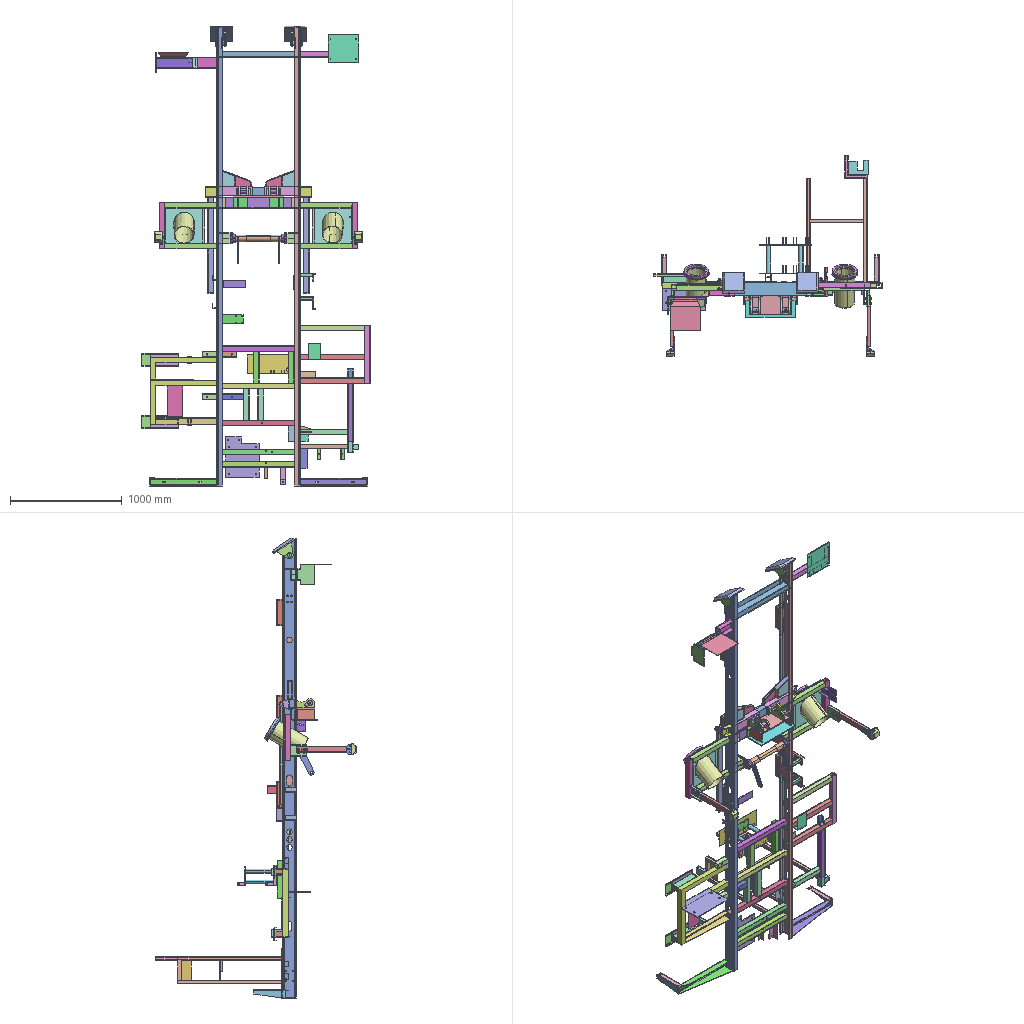Assembly | SolidWorks | 152 different items | 310 placed | box 2045 x 1800 x 4124 mm
Parts list (item | name | quantity | parent item | size | volume | features):
1 | (subassembly) | x1 | - | 650 x 415 x 555 mm | 2554189 mm3 | -
2 | (subassembly) | x1 | - | 625 x 50 x 1040 mm | 1628220 mm3 | -
3 | (subassembly) | x2 | in 20 | 255 x 100 x 75 mm | 251400 mm3 | -
4 | (subassembly) | x1 | - | 75 x 280 x 45 mm | 137505 mm3 | -
5 | (subassembly) | x1 | - | 75 x 280 x 45 mm | 137505 mm3 | -
6 | (subassembly) | x2 | - | 100 x 145 x 100 mm | 200705 mm3 | -
7 | (subassembly) | x1 | - | 320 x 140 x 260 mm | 518000 mm3 | -
8 | (subassembly) | x6 | - | 50 x 55 x 340 mm | 668931 mm3 | -
9 | (subassembly) | x1 | - | 470 x 410 x 340 mm | 1561972 mm3 | features CompositeCurve 1
10 | (subassembly) | x8 | in 12 | 30 x 70 x 30 mm | 19249 mm3 | -
11 | (subassembly) | x1 | - | 100 x 120 x 206 mm | 195480 mm3 | -
12 | (subassembly) | x2 | in 9 | 470 x 170 x 75 mm | 476496 mm3 | -
13 | (subassembly) | x2 | - | 220 x 200 x 152.25 mm | 1422788 mm3 | -
14 | (subassembly) | x1 | - | 740 x 271 x 356.521 mm | 7282688 mm3 | -
15 | (subassembly) | x1 | - | 100 x 120 x 186 mm | 156515 mm3 | -
16 | (subassembly) | x1 | in 1 | 115 x 70 x 590 mm | 694162 mm3 | -
17 | (subassembly) | x1 | - | 115 x 70 x 590 mm | 694162 mm3 | -
18 | (subassembly) | x1 | - | 240 x 550.386 x 1140 mm | 2006489 mm3 | -
19 | (subassembly) | x1 | - | 250 x 58 x 520 mm | 854172 mm3 | -
20 | (subassembly) | x1 | - | 670 x 679 x 350 mm | 6681569 mm3 | -
21 | (subassembly) | x1 | - | 183 x 366.464 x 548.536 mm | 871014 mm3 | -
22 | (subassembly) | x2 | - | 100.467 x 200 x 740 mm | 967974 mm3 | -
23 | (subassembly) | x3 | in 1 | 230 x 230 x 340 mm | 1372483 mm3 | -
24 | (subassembly) | x1 | - | 60 x 415 x 515 mm | 1791277 mm3 | -
25 | - | x2 | in 18 | 30 x 30 x 100 mm | 16864 mm3 | features Extrusion 1, ICE 1
26 | - | x1 | in 21 | 43 x 310 x 270 mm | 250121 mm3 | features Extrusion 1, ICE 1
27 | - | x1 | in 20 | 140 x 280 x 83 mm | 150930 mm3 | features Extrusion 1, Fillet 1, ICE 1
28 | - | x1 | in 20 | 390 x 250 x 8 mm | 755753 mm3 | features ICE 2, Extrusion 1
29 | - | x2 | in 11, 15 | 100 x 120 x 6 mm | 72000 mm3 | features Extrusion 1
30 | - | x1 | in 15 | 180 x 80 x 6 mm | 84515 mm3 | features Extrusion 1, ICE 1
31 | - | x2 | in 20 | 70 x 30 x 100 mm | 55604 mm3 | features Extrusion 1, ICE 1, Shell 1
32 | - | x1 | - | 50 x 120 x 4120 mm | 4129242 mm3 | features ICE 5, Cut 2, Extrusion 1
33 | - | x1 | - | 50 x 120 x 4120 mm | 4181068 mm3 | features ICE 4, Cut 2, Extrusion 1
34 | - | x1 | - | 60 x 60 x 470 mm | 1026298 mm3 | features ICE 2, RevCut 2, Extrusion 1
35 | - | x2 | - | 75 x 75 x 25 mm | 32210 mm3 | features Chamfer 1, Extrusion 1, ICE 1
36 | - | x1 | - | 50 x 50 x 160 mm | 46324 mm3 | features Extrusion 1, ICE 1
37 | - | x2 | - | 25 x 25 x 90 mm | 18731 mm3 | features ICE 4, Chamfer 3, Extrusion 1
38 | - | x2 | - | 77.5 x 50 x 90 mm | 116974 mm3 | features ICE 3, Extrusion 1
39 | - | x2 | - | 67.801 x 45 x 103 mm | 100967 mm3 | features ICE 3, Extrusion 1
40 | - | x2 | in 16, 17 | 105 x 30 x 140 mm | 154453 mm3 | features Extrusion 1, ICE 1
41 | - | x2 | in 16, 17 | 50 x 30 x 450 mm | 193179 mm3 | features ICE 2, Extrusion 1
42 | - | x2 | in 16, 17 | 90 x 135 x 60 mm | 111719 mm3 | features ICE 6, Extrusion 1
43 | - | x2 | in 16, 17 | 100 x 40 x 70 mm | 234811 mm3 | features Extrusion 1, Fillet 1
44 | - | x2 | - | 243.637 x 59.938 x 8 mm | 90831 mm3 | features Extrusion 1, ICE 1
45 | - | x4 | in 14 | 85.082 x 170 x 15 mm | 155113 mm3 | features ICE 3, Extrusion 1
46 | - | x2 | - | 50 x 50 x 280 mm | 157920 mm3 | features Extrusion 1
47 | - | x1 | - | 30 x 30 x 100 mm | 11600 mm3 | features Extrusion 1
48 | - | x1 | - | 50 x 50 x 130 mm | 72524 mm3 | features Cut 1, Extrusion 1
49 | - | x1 | - | 50 x 50 x 190 mm | 106364 mm3 | features Cut 1, Extrusion 1
50 | - | x2 | - | 50 x 50 x 130 mm | 72524 mm3 | features Cut 1, Extrusion 1
51 | - | x2 | - | 45 x 45 x 50 mm | 31416 mm3 | features ICE 2, Extrusion 1
52 | - | x4 | - | 57.32 x 20.473 x 17.73 mm | 7614 mm3 | features RevCut 3, Boss 1, Chamfer 1, Extrusion 1, Fillet 1, LPattern 1
53 | - | x4 | - | 41.4 x 18.475 x 16 mm | 4135 mm3 | features RevCut 3, Boss 1, Chamfer 1, Extrusion 1, Fillet 1, LPattern 1
54 | - | x4 | - | 20.785 x 18 x 10.8 mm | 1984 mm3 | features RevCut 2, Chamfer 1, Extrusion 1, LPattern 1
55 | - | x8 | - | 37.68 x 20.473 x 17.73 mm | 5450 mm3 | features RevCut 3, Boss 1, Chamfer 1, Extrusion 1, Fillet 1, LPattern 1
56 | - | x4 | - | 24 x 24 x 2.5 mm | 799.143 mm3 | features Extrusion 1
57 | - | x4 | - | 50 x 50 x 10 mm | 24215 mm3 | features Extrusion 1
58 | - | x1 | - | 595 x 120 x 70 mm | 542052 mm3 | features ICE 3, Fillet 2, Extrusion 1, Shell 1
59 | - | x1 | - | 595 x 120 x 70 mm | 542052 mm3 | features ICE 3, Fillet 2, Extrusion 1, Shell 1
60 | - | x1 | in 19 | 50 x 50 x 520 mm | 293280 mm3 | features Extrusion 1
61 | - | x1 | in 19 | 270 x 250 x 8 mm | 538392 mm3 | features Cut 1, Extrusion 1
62 | - | x4 | in 19 | 100 x 30 x 5 mm | 7500 mm3 | features Extrusion 1
63 | - | x2 | in 19 | 50 x 30 x 5 mm | 3750 mm3 | features Extrusion 1
64 | - | x1 | in 14 | 90 x 600 x 5 mm | 270000 mm3 | features Extrusion 1, ICE 1
65 | - | x1 | - | 50 x 180 x 10 mm | 87345 mm3 | features Extrusion 1, ICE 1
66 | - | x1 | - | 60 x 140 x 8 mm | 67200 mm3 | features Extrusion 1
67 | - | x1 | in 20 | 595 x 605 x 50 mm | 4237500 mm3 | features ICE 10, Cut 1, Extrusion 1
68 | - | x1 | in 20 | 545 x 80 x 60 mm | 449625 mm3 | features Extrusion 1, ICE 1, Shell 1
69 | - | x1 | - | 45 x 110 x 79.839 mm | 29548 mm3 | features Extrusion 1, ICE 1
70 | - | x1 | - | 79.839 x 110 x 45 mm | 29548 mm3 | features Fillet 2, Extrusion 1
71 | - | x1 | - | 53 x 120 x 740 mm | 751500 mm3 | features ICE 3, Extrusion 1
72 | - | x1 | in 21 | 100 x 50 x 175 mm | 166250 mm3 | features Extrusion 1
73 | - | x1 | in 21 | 43.536 x 90 x 100 mm | 52249 mm3 | features ICE 2, Extrusion 1
74 | - | x1 | in 21 | 70.878 x 56.464 x 5 mm | 9823 mm3 | features Extrusion 1, ICE 1
75 | - | x1 | - | 120 x 120 x 10 mm | 138691 mm3 | features Extrusion 1
76 | - | x1 | in 21 | 100 x 30 x 360 mm | 264321 mm3 | features Extrusion 1, ICE 1
77 | - | x2 | in 22 | 50 x 120 x 125 mm | 108750 mm3 | features Cut 3, Extrusion 1, ICE 1
78 | - | x6 | in 22 | 50 x 120 x 125 mm | 108750 mm3 | features Cut 3, Extrusion 1, ICE 1
79 | - | x6 | in 22 | 90 x 110 x 10 mm | 91931 mm3 | features ICE 2, Extrusion 1
80 | - | x4 | in 22 | 100 x 200 x 10 mm | 174555 mm3 | features ICE 4, Extrusion 1
81 | - | x3 | in 23 | 180 x 180 x 320 mm | 879646 mm3 | features Extrusion 1
82 | - | x3 | in 23 | 230 x 230 x 15 mm | 115846 mm3 | features ICE 5, Cut 1, Extrusion 1
83 | - | x4 | in 1, 24 | 50 x 50 x 465 mm | 262260 mm3 | features Extrusion 1
84 | - | x2 | in 1, 24 | 50 x 50 x 415 mm | 234060 mm3 | features Extrusion 1
85 | - | x2 | in 1, 24 | 400 x 365 x 5 mm | 558599 mm3 | features Extrusion 1, ICE 1
86 | - | x1 | in 11 | 200 x 100 x 70 mm | 123480 mm3 | features Extrusion 1
87 | - | x2 | in 1, 24 | 380 x 330 x 5 mm | 474099 mm3 | features Cut 1, Extrusion 1, ICE 1
88 | - | x2 | in 14 | 100 x 120 x 10 mm | 120000 mm3 | features ICE 3, Extrusion 1
89 | - | x1 | - | 100 x 50 x 100 mm | 84600 mm3 | features ICE 3, Extrusion 1
90 | - | x2 | - | 110 x 100 x 5 mm | 38408 mm3 | features ICE 5, Extrusion 1
91 | - | x2 | - | 65 x 65 x 50 mm | 86394 mm3 | features Extrusion 1
92 | - | x1 | in 7 | 70 x 30 x 260 mm | 185360 mm3 | features Cut 1, Extrusion 1
93 | - | x1 | in 7 | 110 x 30 x 180 mm | 190080 mm3 | features Extrusion 1
94 | - | x4 | in 7 | 30 x 30 x 110 mm | 35640 mm3 | features Cut 1, Extrusion 1
95 | - | x1 | in 1 | 130 x 180 x 28 mm | 68749 mm3 | features ICE 2, Extrusion 1
96 | - | x1 | in 2 | 50 x 50 x 520 mm | 293280 mm3 | features Cut 1, Extrusion 1, ICE 1
97 | - | x1 | in 18 | 240 x 540 x 940 mm | 1507680 mm3 | features ICE 4, Extrusion 1
98 | - | x1 | in 2 | 50 x 50 x 425 mm | 239700 mm3 | features Cut 1, Extrusion 1, ICE 1
99 | - | x2 | in 2 | 50 x 50 x 575 mm | 324300 mm3 | features Cut 1, Extrusion 1
100 | - | x1 | in 2 | 80 x 50 x 50 mm | 27360 mm3 | features Extrusion 1, Shell 1
101 | - | x1 | in 2 | 170 x 60 x 8 mm | 78676 mm3 | features Extrusion 1, ICE 1
102 | - | x1 | in 2 | 50 x 50 x 520 mm | 293280 mm3 | features ICE 2, Extrusion 1
103 | - | x1 | in 2 | 50 x 50 x 575 mm | 324300 mm3 | features Extrusion 1, ICE 1
104 | - | x1 | in 2 | 60 x 70 x 10 mm | 42000 mm3 | features Extrusion 1
105 | - | x1 | in 2 | 140 x 60 x 10 mm | 84000 mm3 | features Extrusion 1
106 | - | x4 | in 3 | 255 x 70 x 3 mm | 53550 mm3 | features Extrusion 1
107 | - | x4 | in 3 | 40 x 70 x 3 mm | 8400 mm3 | features Extrusion 1
108 | - | x1 | in 18 | 80 x 180 x 8 mm | 115200 mm3 | features Extrusion 1
109 | - | x2 | in 3 | 255 x 100 x 5 mm | 127500 mm3 | features ICE 3, Extrusion 1
110 | - | x2 | in 4, 5 | 75 x 280 x 5 mm | 83125 mm3 | features Extrusion 1
111 | - | x2 | in 4, 5 | 8.684 x 279.845 x 40 mm | 54380 mm3 | features ICE 2, Extrusion 1
112 | - | x1 | in 21 | 180 x 155 x 5 mm | 128250 mm3 | features Extrusion 1, ICE 1
113 | - | x2 | - | 54.442 x 50 x 920.099 mm | 408787 mm3 | features ICE 4, Extrusion 1
114 | - | x2 | in 6 | 100 x 60 x 100 mm | 126908 mm3 | features Fillet 2, Extrusion 1, Shell 1
115 | - | x4 | in 6 | 80 x 85 x 8 mm | 36899 mm3 | features Extrusion 1
116 | - | x2 | in 20 | 120 x 20 x 330 mm | 236877 mm3 | features Extrusion 1, ICE 1
117 | - | x1 | in 14 | 80 x 60 x 740 mm | 962000 mm3 | features ICE 6, Cut 2, Extrusion 1
118 | - | x1 | - | 50 x 50 x 740 mm | 402309 mm3 | features ICE 6, Cut 3, Extrusion 1
119 | - | x1 | in 18 | 200 x 30 x 200 mm | 119880 mm3 | features Extrusion 1, ICE 1, Shell 1
120 | - | x1 | - | 50 x 50 x 740 mm | 401838 mm3 | features ICE 11, Cut 4, Extrusion 1
121 | - | x1 | - | 50 x 50 x 740 mm | 402309 mm3 | features ICE 8, Cut 3, Extrusion 1
122 | - | x1 | - | 50 x 50 x 740 mm | 402780 mm3 | features ICE 5, Extrusion 1
123 | - | x1 | - | 50 x 50 x 740 mm | 402780 mm3 | features ICE 5, Extrusion 1
124 | - | x6 | in 8 | 340 x 50 x 5 mm | 85000 mm3 | features Extrusion 1
125 | - | x6 | in 8 | 50 x 50 x 240 mm | 583931 mm3 | features ICE 2, Extrusion 1, Fillet 1
126 | - | x3 | in 23 | 220 x 220 x 30 mm | 376991 mm3 | features Extrusion 1
127 | - | x2 | - | 40 x 40 x 100 mm | 37500 mm3 | features Extrusion 1
128 | - | x2 | in 12 | 470 x 170 x 5 mm | 399500 mm3 | features Extrusion 1
129 | - | x16 | in 10 | 30 x 70 x 5 mm | 9624 mm3 | features Extrusion 1
130 | - | x1 | in 18 | 180 x 130 x 5 mm | 86000 mm3 | features Extrusion 1
131 | - | x2 | in 9 | 50 x 50 x 340 mm | 191760 mm3 | features Extrusion 1
132 | - | x2 | in 9 | 50 x 30 x 170 mm | 53040 mm3 | features Extrusion 1, ICE 1
133 | - | x2 | in 9 | 40 x 40 x 250 mm | 59690 mm3 | features Extrusion 1
134 | - | x1 | - | 300 x 360 x 10 mm | 979288 mm3 | features ICE 2, Extrusion 1
135 | - | x2 | in 13 | 220 x 200 x 30 mm | 1200000 mm3 | features ICE 1, NetBlend 1
136 | - | x4 | in 13 | 160 x 10 x 122.25 mm | 111394 mm3 | features Extrusion 1, ICE 1
137 | - | x2 | in 14 | 154.478 x 150 x 8 mm | 150374 mm3 | features Extrusion 1
138 | - | x2 | in 14 | 88 x 76 x 318 mm | 396864 mm3 | features ICE 3, Extrusion 1
139 | - | x2 | in 14 | 300 x 150 x 8 mm | 227361 mm3 | features Extrusion 1
140 | - | x1 | in 14 | 308 x 158.521 x 50 mm | 106428 mm3 | features Extrusion 1, ICE 1
141 | - | x1 | in 18 | 120 x 240 x 5 mm | 144000 mm3 | features Extrusion 1
142 | - | x1 | in 14 | 308 x 158.521 x 50 mm | 106428 mm3 | features Extrusion 1, ICE 1
143 | - | x2 | in 14 | 320 x 80 x 8 mm | 197260 mm3 | features Extrusion 1, ICE 1
144 | - | x2 | in 14 | 137.522 x 90.425 x 8 mm | 71106 mm3 | features Extrusion 1
145 | - | x2 | in 14 | 8 x 93.358 x 42 mm | 30876 mm3 | features Extrusion 1, ICE 1
146 | - | x4 | in 14 | 150 x 90 x 10 mm | 135000 mm3 | features Extrusion 1
147 | - | x1 | in 14 | 440 x 180 x 10 mm | 792000 mm3 | features Extrusion 1
148 | - | x1 | in 14 | 460 x 240 x 10 mm | 1004000 mm3 | features ICE 2, Extrusion 1
149 | - | x2 | in 14 | 20 x 60 x 10 mm | 12000 mm3 | features ICE 2, Extrusion 1
150 | - | x4 | in 14 | 20 x 70 x 10 mm | 14000 mm3 | features Extrusion 1
151 | - | x1 | - | 150 x 60 x 110 mm | 112750 mm3 | features Extrusion 1
152 | - | x1 | in 14 | 100 x 48 x 740 mm | 683700 mm3 | features ICE 6, Cut 4, Extrusion 1
Mates (type | each side: item.copy, entity, surface, feature):
In the top assembly
Coincident | 32.1 face plane Boss-Extrude 1 | 33.1 face plane Boss-Extrude 1 | 2 times
Coincident | 32.1 face plane Boss-Extrude 1 | 118.1 face plane Cut-Extrude 1
Coincident | 118.1 face plane Boss-Extrude 1 | 36.1 face plane Boss-Extrude 1 | 2 times
DistanceDim | 118.1 face plane Boss-Extrude 1 | 32.1 face plane Boss-Extrude 1
Coincident | 36.1 face plane Boss-Extrude 1 | 57.1 face plane Boss-Extrude 1
Concentric | 36.1 face cylinder Cut-Extrude 1 | 57.1 face cylinder Boss-Extrude 1
Parallel | 36.1 face plane Boss-Extrude 1 | 57.1 face plane Boss-Extrude 1
DistanceDim | 36.1 face plane Boss-Extrude 1 | 32.1 face plane Boss-Extrude 1
Coincident | 118.1 face plane Boss-Extrude 1 | 47.1 face plane Boss-Extrude 2 | 2 times
DistanceDim | 57.2 face plane Boss-Extrude 1 | 32.1 face plane Boss-Extrude 1
Coincident | 32.1 face plane Boss-Extrude 1 | 57.3 face plane Boss-Extrude 1 | 2 times
Coincident | 118.1 face plane Boss-Extrude 1 | 134.1 face plane Boss-Extrude 1
Coincident | 32.1 face plane Boss-Extrude 1 | 120.1 face plane Cut-Extrude 1
DistanceDim | 120.1 face plane Boss-Extrude 1 | 118.1 face plane Boss-Extrude 1
Coincident | 57.3 face plane Boss-Extrude 1 | 120.1 face plane Boss-Extrude 1
Coincident | 57.2 face plane Boss-Extrude 1 | 120.1 face plane Boss-Extrude 1 | 2 times
DistanceDim | 47.1 face plane Boss-Extrude 2 | 32.1 face plane Boss-Extrude 1
DistanceDim | 134.1 face plane Boss-Extrude 1 | 33.1 face plane Boss-Extrude 1 | 2 times
Coincident | 32.1 face plane Boss-Extrude 1 | 121.1 face plane Cut-Extrude 1
DistanceDim | 120.1 face plane Boss-Extrude 1 | 121.1 face plane Boss-Extrude 1
Coincident | 121.1 face plane Boss-Extrude 1 | 57.4 face plane Boss-Extrude 1
Concentric | 121.1 face cylinder Cut-Extrude 3 | 57.4 face cylinder Boss-Extrude 1
Coincident | 121.1 face plane Boss-Extrude 1 | 66.1 face plane Boss-Extrude 1 | 2 times
Coincident | 32.1 face plane Boss-Extrude 1 | 66.1 face plane Boss-Extrude 1
Coincident | 32.1 face plane Boss-Extrude 1 | 122.1 face plane Cut-Extrude 1
Coincident | 32.1 edge | 122.1 face plane Cut-Extrude 1
DistanceDim | 121.1 face plane Boss-Extrude 1 | 122.1 face plane Boss-Extrude 1
Coincident | 32.1 face plane Boss-Extrude 1 | 123.1 face plane Cut-Extrude 1 | 2 times
DistanceDim | 123.1 face plane Boss-Extrude 1 | 122.1 face plane Boss-Extrude 1
Coincident | 121.1 face plane Boss-Extrude 1 | 46.1 face plane Boss-Extrude 2 | 2 times
Coincident | 122.1 face plane Boss-Extrude 1 | 46.2 face plane Boss-Extrude 2
DistanceDim | 46.1 face plane Boss-Extrude 2 | 33.1 face plane Boss-Extrude 1
DistanceDim | 46.2 face plane Boss-Extrude 2 | 46.1 face plane Boss-Extrude 2
Coincident | 46.1 face plane Boss-Extrude 2 | 49.1 face plane Boss-Extrude 2 | 2 times
Coincident | 33.1 face plane Boss-Extrude 1 | 48.1 face plane Boss-Extrude 1
Coincident | 123.1 face plane Boss-Extrude 1 | 48.1 face plane Boss-Extrude 1 | 2 times
DistanceDim | 49.1 select_type:24 | 48.1 select_type:24
Coincident | 32.1 face plane Boss-Extrude 1 | 121.1 face plane Cut-Extrude 6
Coincident | 121.1 face plane Boss-Extrude 1 | 46.2 face plane Boss-Extrude 2
Coincident | 33.1 face plane Boss-Extrude 1 | 120.1 face plane Boss-Extrude 2
Coincident | 33.1 face plane Boss-Extrude 1 | 121.1 face plane Boss-Extrude 4
Coincident | 32.1 face plane Boss-Extrude 1 | 118.1 face plane Cut-Extrude 6
Coincident | 33.1 face plane Boss-Extrude 1 | 50.1 face plane Boss-Extrude 1
Coincident | 122.1 face plane Boss-Extrude 1 | 50.1 face plane Boss-Extrude 1
Coincident | 49.1 face plane Boss-Extrude 2 | 50.1 face plane Boss-Extrude 1
Coincident | 33.1 face plane Boss-Extrude 1 | 50.2 face plane Boss-Extrude 1
Coincident | 46.2 face plane Boss-Extrude 2 | 65.1 face plane Boss-Extrude 1 | 2 times
DistanceDim | 65.1 face plane Boss-Extrude 1 | 121.1 face plane Boss-Extrude 1
Coincident | 32.1 face plane Boss-Extrude 1 | 152.1 face plane Cut-Extrude 2
Coincident | 32.1 face plane Boss-Extrude 1 | 152.1 face plane Boss-Extrude 4
Coincident | 152.1 face plane Boss-Extrude 1 | assembly select_type:11
Coincident | 33.1 face plane Boss-Extrude 1 | 29.1 face plane Boss-Extrude 1 | 2 times
DistanceDim | 29.1 face plane Boss-Extrude 1 | 123.1 face plane Boss-Extrude 1
Coincident | 33.1 face plane Boss-Extrude 1 | 29.2 face plane Boss-Extrude 1 | 2 times
DistanceDim | 29.2 face plane Boss-Extrude 1 | 123.1 face plane Boss-Extrude 1
Coincident | 32.1 face plane Boss-Extrude 1 | 75.1 face plane Boss-Extrude 1 | 2 times
DistanceDim | 75.1 face plane Boss-Extrude 1 | 123.1 edge
Coincident | 33.1 face plane Boss-Extrude 1 | 78.1 face plane Cut-Extrude 1
Coincident | 32.1 face plane Boss-Extrude 1 | 77.1 face plane Cut-Extrude 1
Coincident | 78.1 face plane Boss-Extrude 1 | 77.1 face plane Boss-Extrude 1
Coincident | 32.1 face plane Boss-Extrude 1 | 71.1 face plane Cut-Extrude 3
Coincident | 33.1 face plane Boss-Extrude 1 | 71.1 face plane Boss-Extrude 1
DistanceDim | 71.1 face plane Boss-Extrude 1 | 32.1 face plane Boss-Extrude 1
Coincident | 48.1 face plane Boss-Extrude 1 | 50.2 face plane Boss-Extrude 1 | 2 times
Coincident | 88.1 face plane Boss-Extrude 1 | 146.1 face plane Boss-Extrude 1
Coincident | 148.1 face plane Boss-Extrude 2 | 146.1 face plane Boss-Extrude 1
Coincident | 148.1 face plane Boss-Extrude 1 | 146.1 face plane Boss-Extrude 1
Coincident | 88.2 face plane Boss-Extrude 1 | 146.2 face plane Boss-Extrude 1
Coincident | 148.1 face plane Boss-Extrude 1 | 146.2 face plane Boss-Extrude 1
Coincident | 148.1 face plane Boss-Extrude 3 | 146.2 face plane Boss-Extrude 1
Coincident | 32.1 face plane Boss-Extrude 1 | 98.1 face plane Boss-Extrude 2
Coincident | 33.1 face plane Boss-Extrude 1 | 67.1 face plane Boss-Extrude 9
Coincident | 33.1 face plane Boss-Extrude 1 | 68.1 face plane Boss-Extrude 1
Coincident | 50.2 face plane Boss-Extrude 1 | 67.1 face plane Boss-Extrude 1
Coincident | 32.1 face plane Boss-Extrude 1 | 98.1 face plane Boss-Extrude 1
DistanceDim | 96.1 face plane Cut-Extrude 1 | 32.1 face plane Boss-Extrude 1
Coincident | 33.1 face plane Boss-Extrude 1 | 59.1 face plane Boss-Extrude 1 | 2 times
DistanceDim | 59.1 face plane Boss-Extrude 1 | 33.1 face plane Boss-Extrude 1
Coincident | 32.1 face plane Boss-Extrude 1 | 58.1 face plane Boss-Extrude 1
DistanceDim | 58.1 face plane Boss-Extrude 1 | 32.1 face plane Boss-Extrude 1
Coincident | 58.1 face plane Boss-Extrude 1 | 32.1 face plane Boss-Extrude 1
Coincident | 59.1 face plane Boss-Extrude 1 | 110.1 face plane Boss-Extrude 3
Coincident | 59.1 face plane Boss-Extrude 1 | 111.1 face plane Boss-Extrude 1
Coincident | 59.1 edge | 110.1 face plane Boss-Extrude 3
Coincident | 58.1 face plane Boss-Extrude 1 | 110.2 face plane Boss-Extrude 3
Coincident | 58.1 face plane Boss-Extrude 1 | 111.2 face plane Boss-Extrude 1
Coincident | 58.1 edge | 110.2 face plane Boss-Extrude 3
Coincident | 33.1 face plane Boss-Extrude 1 | 114.1 face plane Boss-Extrude 1
Parallel | 33.1 face plane Boss-Extrude 1 | 114.1 face plane Boss-Extrude 1
DistanceDim | 114.1 face plane Boss-Extrude 1 | 123.1 face plane Boss-Extrude 1
Coincident | 32.1 face plane Boss-Extrude 1 | 114.2 face plane Boss-Extrude 1
DistanceDim | 114.2 face plane Boss-Extrude 1 | 123.1 face plane Boss-Extrude 1
Coincident | 33.1 face plane Boss-Extrude 1 | 124.1 face plane Boss-Extrude 1
Coincident | 33.1 face plane Boss-Extrude 1 | 125.1 face plane Boss-Extrude 2
Coincident | 33.1 face plane Boss-Extrude 1 | 124.2 face plane Boss-Extrude 1 | 2 times
Coincident | 33.1 face plane Boss-Extrude 1 | 124.3 face plane Boss-Extrude 1 | 2 times
Coincident | 32.1 face plane Boss-Extrude 1 | 124.4 face plane Boss-Extrude 1 | 2 times
Coincident | 32.1 face plane Boss-Extrude 1 | 124.5 face plane Boss-Extrude 1 | 2 times
Coincident | 32.1 face plane Boss-Extrude 1 | 124.6 face plane Boss-Extrude 1 | 2 times
DistanceDim | 124.1 face plane Boss-Extrude 1 | 123.1 face plane Boss-Extrude 1
DistanceDim | 124.2 face plane Boss-Extrude 1 | 123.1 face plane Boss-Extrude 1
DistanceDim | 124.2 face plane Boss-Extrude 1 | 124.3 face plane Boss-Extrude 1
DistanceDim | 124.6 face plane Boss-Extrude 1 | 123.1 face plane Boss-Extrude 1
DistanceDim | 124.5 face plane Boss-Extrude 1 | 123.1 face plane Boss-Extrude 1
DistanceDim | 124.4 face plane Boss-Extrude 1 | 124.5 face plane Boss-Extrude 1
Coincident | 115.1 edge | 113.1 face cylinder Cut-Extrude 2
Coincident | 115.1 face plane Boss-Extrude 1 | 113.1 face plane Boss-Extrude 1
Coincident | 32.1 face plane Boss-Extrude 1 | 83.1 face plane Boss-Extrude 1
Parallel | 32.1 face plane Boss-Extrude 1 | 83.2 face plane Boss-Extrude 1
Coincident | 33.1 face plane Boss-Extrude 1 | 83.3 face plane Boss-Extrude 1
Parallel | 33.1 face plane Boss-Extrude 1 | 83.3 face plane Boss-Extrude 1
Coincident | 115.2 face cylinder Boss-Extrude 1 | 113.2 edge
Coincident | 115.2 face plane Boss-Extrude 1 | 113.2 face plane Boss-Extrude 1
Coincident | 123.1 face plane Boss-Extrude 1 | 131.1 face plane Boss-Extrude 2
DistanceDim | 114.2 face plane Boss-Extrude 1 | 32.1 face plane Boss-Extrude 1
DistanceDim | 33.1 face plane Boss-Extrude 1 | 114.1 face plane Boss-Extrude 1
Coincident | 32.1 face plane Boss-Extrude 1 | 60.1 face plane Boss-Extrude 1 | 2 times
Concentric | 32.1 face cylinder Cut-Extrude 5 | 91.1 face cylinder Boss-Extrude 1
Coincident | 32.1 face plane Boss-Extrude 1 | 91.1 face plane Boss-Extrude 1
Coincident | 51.1 face plane Boss-Extrude 1 | 91.1 face plane Boss-Extrude 1
Concentric | 33.1 face cylinder Cut-Extrude 5 | 91.2 face cylinder Boss-Extrude 1
Coincident | 33.1 face plane Boss-Extrude 1 | 91.2 face plane Boss-Extrude 1
Coincident | 51.2 face plane Boss-Extrude 1 | 91.2 face plane Boss-Extrude 1
Concentric | 51.2 face cylinder Boss-Extrude 2 | 91.2 face cylinder Boss-Extrude 1
Concentric | 51.1 face cylinder Boss-Extrude 2 | 91.1 face cylinder Boss-Extrude 1
Concentric | 51.2 face cylinder Cut-Extrude 2 | 136.1 face cylinder Cut-Extrude 1
Concentric | 51.1 face cylinder Cut-Extrude 2 | 136.2 face cylinder Cut-Extrude 1
Coincident | 32.1 face plane Boss-Extrude 1 | 136.3 face plane Boss-Extrude 1
Coincident | 71.1 face plane Boss-Extrude 1 | 60.1 face plane Boss-Extrude 1
DistanceDim | 131.2 face plane Boss-Extrude 2 | 32.1 face plane Boss-Extrude 1
DistanceDim | 131.2 face plane Boss-Extrude 2 | 123.1 face plane Boss-Extrude 1
DistanceDim | 83.2 face plane Boss-Extrude 1 | 123.1 face plane Boss-Extrude 1
DistanceDim | 83.4 face plane Boss-Extrude 1 | 123.1 face plane Boss-Extrude 1
Coincident | 33.1 face plane Boss-Extrude 1 | 136.1 face plane Boss-Extrude 1
Coincident | 84.1 face plane Boss-Extrude 1 | 40.1 face plane Boss-Extrude 1 | 2 times
Coincident | 33.1 face plane Boss-Extrude 1 | 72.1 face plane Boss-Extrude 1 | 2 times
DistanceDim | 83.2 face plane Boss-Extrude 1 | 32.1 face plane Boss-Extrude 1
DistanceDim | 83.3 face plane Boss-Extrude 1 | 33.1 face plane Boss-Extrude 1
Coincident | 32.1 face plane Boss-Extrude 1 | 99.1 face plane Cut-Extrude 1
DistanceDim | 99.1 face plane Boss-Extrude 1 | 99.2 face plane Boss-Extrude 1
Coincident | 102.1 face plane Boss-Extrude 1 | 99.1 face plane Boss-Extrude 1
Coincident | 98.1 face plane Boss-Extrude 1 | 97.1 face plane Boss-Extrude 1
DistanceDim | 97.1 face plane Boss-Extrude 1 | 32.1 edge
Coincident | 32.1 face plane Boss-Extrude 1 | 94.1 face plane Cut-Extrude 1
DistanceDim | 93.1 face plane Boss-Extrude 1 | 123.1 face plane Boss-Extrude 1
Coincident | 32.1 face plane Boss-Extrude 1 | 94.2 face plane Boss-Extrude 1
Coincident | 99.1 face plane Boss-Extrude 1 | 151.1 face plane Boss-Extrude 1 | 2 times
DistanceDim | 32.1 face plane Boss-Extrude 1 | 151.1 face plane Boss-Extrude 1
Coincident | 32.1 face plane Boss-Extrude 1 | 90.1 face plane Boss-Extrude 1
Concentric | 91.1 face cylinder Boss-Extrude 1 | 90.1 face cylinder Cut-Extrude 1
Coincident | 32.1 face plane Boss-Extrude 1 | 90.1 face plane Cut-Extrude 2
Coincident | 33.1 face plane Boss-Extrude 1 | 90.2 face plane Boss-Extrude 1
Concentric | 91.2 face cylinder Boss-Extrude 1 | 90.2 face cylinder Cut-Extrude 1
Coincident | 33.1 face plane Boss-Extrude 1 | 90.2 face plane Cut-Extrude 3
Coincident | 33.1 edge | 69.1 face plane Boss-Extrude 2
Coincident | 33.1 face plane Boss-Extrude 1 | 69.1 face plane Boss-Extrude 2
Coincident | 33.1 vertex | 69.1 vertex
Coincident | 32.1 face plane Boss-Extrude 1 | 70.1 face plane Boss-Extrude 1 | 2 times
Coincident | 32.1 vertex | 70.1 vertex
Coincident | 32.1 face plane Boss-Extrude 1 | 97.1 face plane Boss-Extrude 1
Coincident | 80.1 face plane Boss-Extrude 1 | 35.1 face plane Boss-Extrude 1
Concentric | 34.1 face cylinder Cut-Extrude 1 | 35.2 face cylinder Boss-Extrude 1
Concentric | 34.1 face cylinder Cut-Extrude 2 | 35.1 face cylinder Boss-Extrude 1
Coincident | 34.1 face plane Boss-Extrude 1 | 35.1 face plane Boss-Extrude 1
Coincident | 34.1 face plane Boss-Extrude 1 | 35.2 face plane Boss-Extrude 1
Coincident | 33.1 face plane Boss-Extrude 1 | 77.2 face plane Cut-Extrude 2
Coincident | 32.1 face plane Boss-Extrude 1 | 78.2 face plane Cut-Extrude 2
Coincident | 41.1 face plane Boss-Extrude 1 | 52.1 face plane BaseHead | 2 times
Concentric | 41.2 face cylinder Cut-Extrude 2 | 52.2 face cylinder BaseBody | 2 times
Coincident | 41.2 face plane Boss-Extrude 1 | 52.2 face plane BaseHead | 2 times
Coincident | 41.2 face plane Boss-Extrude 1 | 52.3 face plane BaseHead | 2 times
Concentric | 41.2 face cylinder Cut-Extrude 3 | 52.3 face cylinder BaseBody
Concentric | 41.1 face cylinder Cut-Extrude 2 | 52.1 face cylinder BaseBody
Concentric | 41.1 face cylinder Cut-Extrude 3 | 52.4 face cylinder BaseBody
Coincident | 41.1 face plane Boss-Extrude 1 | 52.4 face plane BaseHead
Concentric | 52.4 face cylinder BaseBody | 54.1 face cylinder BaseNut
Concentric | 52.1 face cylinder BaseBody | 54.2 face cylinder BaseNut
Coincident | 40.1 face plane Boss-Extrude 1 | 56.1 face plane Base-Extrude | 2 times
Concentric | 52.2 face cylinder BaseBody | 56.2 face cylinder Base-Extrude
Concentric | 52.3 face cylinder BaseBody | 56.3 face cylinder Base-Extrude
Concentric | 52.2 face cylinder BaseBody | 54.3 edge
Concentric | 52.3 face cylinder BaseBody | 54.4 edge
Coincident | 40.2 face plane Boss-Extrude 1 | 56.2 face plane Base-Extrude
Coincident | 54.3 face plane BaseNut | 56.2 face plane Base-Extrude
Coincident | 40.2 face plane Boss-Extrude 1 | 56.3 face plane Base-Extrude
Coincident | 54.4 face plane BaseNut | 56.3 face plane Base-Extrude
Concentric | 52.1 face cylinder BaseBody | 56.1 face cylinder Base-Extrude
Coincident | 54.2 face plane BaseNut | 56.1 face plane Base-Extrude
Concentric | 52.4 face cylinder BaseBody | 56.4 face cylinder Base-Extrude
Coincident | 40.1 face plane Boss-Extrude 1 | 56.4 face plane Base-Extrude
Coincident | 54.1 face plane BaseNut | 56.4 face plane Base-Extrude
Concentric | 115.2 edge | 37.1 face cylinder Boss-Extrude 2
Concentric | 113.1 face cylinder Boss-Extrude 2 | 37.2 face cylinder Boss-Extrude 2
Concentric | 51.1 face cylinder Cut-Extrude 2 | 39.1 face cylinder Boss-Extrude 1
Coincident | 136.3 face plane Boss-Extrude 1 | 39.1 face plane Boss-Extrude 3
Concentric | 51.2 face cylinder Cut-Extrude 2 | 39.2 face cylinder Boss-Extrude 1
Coincident | 136.1 face plane Boss-Extrude 1 | 39.2 face plane Boss-Extrude 3
Concentric | 45.1 face cylinder Boss-Extrude 1 | 38.1 face cylinder Boss-Extrude 1
Coincident | 45.1 face plane Boss-Extrude 1 | 38.1 face plane Boss-Extrude 2
Concentric | 45.2 face cylinder Boss-Extrude 1 | 38.2 face cylinder Boss-Extrude 1
Coincident | 45.2 face plane Boss-Extrude 4 | 38.2 face plane Boss-Extrude 2
Concentric | 80.2 face cylinder Cut-Extrude 1 | 55.1 face cylinder BaseBody
Coincident | 80.2 face plane Boss-Extrude 1 | 55.1 face plane BaseHead
Concentric | 80.2 face cylinder Cut-Extrude 1 | 55.2 face cylinder BaseBody
Coincident | 80.2 face plane Boss-Extrude 1 | 55.2 face plane BaseHead
Concentric | 80.2 face cylinder Cut-Extrude 1 | 55.3 face cylinder BaseBody
Coincident | 80.2 face plane Boss-Extrude 1 | 55.3 face plane BaseHead
Concentric | 80.2 face cylinder Cut-Extrude 1 | 55.4 face cylinder BaseBody
Coincident | 80.2 face plane Boss-Extrude 1 | 55.4 face plane BaseHead
Concentric | 80.1 face cylinder Cut-Extrude 1 | 55.5 face cylinder BaseBody
Coincident | 80.1 face plane Boss-Extrude 1 | 55.5 face plane BaseHead
Concentric | 80.1 face cylinder Cut-Extrude 1 | 55.6 face cylinder BaseBody
Coincident | 80.1 face plane Boss-Extrude 1 | 55.6 face plane BaseHead
Concentric | 80.1 face cylinder Cut-Extrude 1 | 55.7 face cylinder BaseBody
Coincident | 80.1 face plane Boss-Extrude 1 | 55.7 face plane BaseHead
Concentric | 80.1 face cylinder Cut-Extrude 1 | 55.8 face cylinder BaseBody
Coincident | 80.1 face plane Boss-Extrude 1 | 55.8 face plane BaseHead
PlanarAngleDim | 82.1 face plane Boss-Extrude 1 | 87.1 face plane Boss-Extrude 1
PlanarAngleDim | 82.2 face plane Boss-Extrude 1 | 87.2 face plane Boss-Extrude 1
Concentric | 34.1 face cylinder Boss-Extrude 1 | 44.1 face cylinder Boss-Extrude 1
Concentric | 34.1 face cylinder Boss-Extrude 1 | 44.2 face cylinder Boss-Extrude 1
DistanceDim | 44.1 face plane Boss-Extrude 1 | 32.1 face plane Boss-Extrude 1
DistanceDim | 44.2 face plane Boss-Extrude 1 | 33.1 face plane Boss-Extrude 1
DistanceDim | 78.1 face plane Boss-Extrude 1 | 58.1 face plane Boss-Extrude 1
Coincident | 44.1 face plane Boss-Extrude 1 | 44.2 face plane Boss-Extrude 1
Coincident | 135.1 face plane 边界1 | 135.2 face plane 边界1
Parallel | 135.1 face plane Boss-Extrude 2 | 70.1 face plane Boss-Extrude 1
DistanceDim | 72.1 face plane Boss-Extrude 1 | 33.1 edge
Coincident | 33.1 face plane Boss-Extrude 1 | 127.1 face plane Boss-Extrude 1
DistanceDim | 50.2 face plane Boss-Extrude 1 | 127.1 face plane Boss-Extrude 1
Coincident | 33.1 face plane Boss-Extrude 1 | 127.2 face plane Boss-Extrude 1
DistanceDim | 127.2 face plane Boss-Extrude 1 | 127.1 face plane Boss-Extrude 1
DistanceDim | 40.1 face plane Boss-Extrude 1 | 83.4 face plane Boss-Extrude 1
Concentric | 42.1 face cylinder Cut-Extrude 4 | 53.1 face cylinder BaseBody
Concentric | 42.1 face cylinder Cut-Extrude 3 | 53.2 face cylinder BaseBody
DistanceDim | 43.1 face plane Boss-Extrude 1 | 53.2 face plane BaseBody
DistanceDim | 53.1 face plane BaseBody | 43.1 face plane Boss-Extrude 1
Concentric | 42.2 face cylinder Cut-Extrude 3 | 53.3 face cylinder BaseBody
Concentric | 42.2 face cylinder Cut-Extrude 4 | 53.4 face cylinder BaseBody
DistanceDim | 53.3 face plane BaseBody | 43.2 face plane Boss-Extrude 1
DistanceDim | 53.4 face plane BaseBody | 43.2 face plane Boss-Extrude 1
DistanceDim | 127.1 face plane Boss-Extrude 1 | 33.1 face plane Boss-Extrude 1
Coincident | 98.1 face plane Boss-Extrude 1 | 62.1 face plane Boss-Extrude 1
Coincident | 32.1 face plane Boss-Extrude 1 | 62.1 face plane Boss-Extrude 1
Coincident | 98.1 face plane Boss-Extrude 1 | 62.2 face plane Boss-Extrude 1
Coincident | 32.1 face plane Boss-Extrude 1 | 62.2 face plane Boss-Extrude 1
Concentric | 80.1 face cylinder Boss-Extrude 1 | 35.1 face cylinder Boss-Extrude 1
Coincident | 96.1 face plane Boss-Extrude 1 | 89.1 face plane Boss-Extrude 1 | 2 times
Coincident | 96.1 face plane Cut-Extrude 1 | 89.1 face plane Cut-Extrude 1
In subassembly 11
Coincident | 29.3 face plane Boss-Extrude 1 | 86.1 face plane Boss-Extrude 1 | 3 times
In subassembly 14
Coincident | 152.2 face plane Boss-Extrude 1 | 64.1 face plane Boss-Extrude 1
Coincident | 147.1 face plane Boss-Extrude 1 | 88.3 face plane Boss-Extrude 1 | 2 times
Coincident | 147.1 face plane Boss-Extrude 1 | 88.4 face plane Boss-Extrude 1 | 2 times
Coincident | 147.1 face plane Boss-Extrude 1 | 88.4 face plane Cut-Extrude 1
Coincident | 147.1 face plane Boss-Extrude 1 | 88.3 face plane Cut-Extrude 1
Coincident | 147.1 face plane Boss-Extrude 1 | 152.2 face plane Boss-Extrude 1
Coincident | 148.2 face plane Boss-Extrude 1 | 117.1 face plane Boss-Extrude 1 | 2 times
Coincident | 152.2 face plane Boss-Extrude 1 | 148.2 face plane Boss-Extrude 1
Coincident | 148.2 face plane Boss-Extrude 1 | 45.3 face plane Boss-Extrude 1
Coincident | 148.2 face plane Boss-Extrude 1 | 45.4 face plane Boss-Extrude 1
Coincident | 148.2 face plane Boss-Extrude 1 | 45.5 face plane Boss-Extrude 1
Coincident | 148.2 face plane Boss-Extrude 1 | 45.6 face plane Boss-Extrude 1
DistanceDim | 45.6 face plane Boss-Extrude 1 | 148.2 face plane Boss-Extrude 3
Coincident | 148.2 select_type:25 | 117.1 select_type:25
Coincident | 147.1 select_type:24 | 152.2 select_type:24
Coincident | 152.2 select_type:25 | 148.2 select_type:24
DistanceDim | 45.6 face plane Boss-Extrude 1 | 45.5 face plane Boss-Extrude 4
DistanceDim | 45.3 face plane Boss-Extrude 4 | 45.4 face plane Boss-Extrude 1
DistanceDim | 45.3 face plane Boss-Extrude 4 | 148.2 face plane Boss-Extrude 2
DistanceDim | 64.1 face plane Boss-Extrude 1 | 152.2 face plane Boss-Extrude 5
Parallel | 152.2 face plane Boss-Extrude 1 | 117.1 face plane Boss-Extrude 1
Coincident | 117.1 face plane Boss-Extrude 1 | 138.1 face plane Boss-Extrude 1 | 2 times
Coincident | 117.1 face plane Boss-Extrude 1 | 138.2 face plane Boss-Extrude 1 | 2 times
Coincident | 152.2 face plane Cut-Extrude 1 | 138.2 face plane Boss-Extrude 1
Coincident | 45.3 face plane Boss-Extrude 1 | 138.2 face plane Boss-Extrude 1
Coincident | 45.4 face plane Boss-Extrude 1 | 138.2 face plane Boss-Extrude 1
Coincident | 45.5 face plane Boss-Extrude 1 | 138.1 face plane Boss-Extrude 1
Coincident | 45.6 face plane Boss-Extrude 1 | 138.1 face plane Boss-Extrude 1
Coincident | 138.2 face plane Boss-Extrude 1 | 139.1 face plane Boss-Extrude 2
Coincident | 138.1 face plane Boss-Extrude 1 | 139.2 face plane Boss-Extrude 2
Coincident | 117.1 face plane Boss-Extrude 2 | 138.1 face plane Boss-Extrude 2
Coincident | 138.1 face plane Boss-Extrude 2 | 139.2 face plane Boss-Extrude 2
Coincident | 139.1 face plane Boss-Extrude 2 | 140.1 face plane Boss-Extrude 1 | 2 times
Concentric | 139.1 face cylinder Boss-Extrude 2 | 140.1 face cylinder Boss-Extrude 1
Coincident | 139.2 face plane Boss-Extrude 2 | 142.1 face plane Boss-Extrude 1 | 2 times
Concentric | 139.2 face cylinder Boss-Extrude 2 | 142.1 face cylinder Boss-Extrude 1
Coincident | 117.1 face plane Boss-Extrude 3 | 138.2 face plane Boss-Extrude 3
Coincident | 138.2 edge | 139.1 face plane Boss-Extrude 2
Coincident | 138.2 face plane Boss-Extrude 3 | 139.1 face plane Boss-Extrude 2
Coincident | 138.1 face plane Boss-Extrude 4 | 139.2 face plane Boss-Extrude 2
Coincident | 117.1 face plane Boss-Extrude 1 | 143.1 face plane Boss-Extrude 1
Coincident | 138.2 face plane Boss-Extrude 1 | 143.1 face plane Boss-Extrude 1
Coincident | 117.1 face plane Boss-Extrude 3 | 143.1 face plane Boss-Extrude 1
Coincident | 148.2 face plane Boss-Extrude 1 | 143.2 face plane Boss-Extrude 1
Coincident | 138.1 face plane Boss-Extrude 2 | 143.2 face plane Boss-Extrude 1
Coincident | 138.1 face plane Boss-Extrude 1 | 143.2 face plane Boss-Extrude 1
Coincident | 140.1 face plane Cut-Extrude 1 | 144.1 face plane Boss-Extrude 1
Coincident | 142.1 face plane Cut-Extrude 2 | 144.2 face plane Boss-Extrude 1
Coincident | 138.1 face plane Boss-Extrude 1 | 144.2 face plane Boss-Extrude 1
Coincident | 142.1 face plane Boss-Extrude 1 | 144.2 face plane Boss-Extrude 1
Coincident | 140.1 face plane Boss-Extrude 1 | 144.1 face plane Boss-Extrude 1
Coincident | 138.2 face plane Boss-Extrude 1 | 144.1 face plane Boss-Extrude 1
Coincident | 138.2 face plane Boss-Extrude 1 | 145.1 face plane Boss-Extrude 1
Parallel | 144.1 face plane Boss-Extrude 1 | 145.1 face plane Boss-Extrude 1
Coincident | 144.1 face plane Boss-Extrude 1 | 145.1 face plane Boss-Extrude 1
Coincident | 140.1 face plane Boss-Extrude 1 | 137.1 face plane Boss-Extrude 1 | 3 times
Coincident | 139.1 face plane Boss-Extrude 2 | 145.1 face plane Boss-Extrude 2
Coincident | 138.1 face plane Boss-Extrude 1 | 145.2 face plane Boss-Extrude 1
Coincident | 139.2 face plane Boss-Extrude 2 | 145.2 face plane Boss-Extrude 1
Coincident | 144.2 face plane Boss-Extrude 1 | 145.2 face plane Boss-Extrude 1
Coincident | 138.1 face plane Boss-Extrude 1 | 137.2 face plane Boss-Extrude 1
Coincident | 145.2 face plane Boss-Extrude 2 | 137.2 face plane Boss-Extrude 1
Coincident | 138.1 edge | 137.2 face plane Boss-Extrude 1
Coincident | 45.3 face plane Boss-Extrude 4 | 150.1 face plane Boss-Extrude 1
Coincident | 138.2 face plane Boss-Extrude 1 | 150.1 face plane Boss-Extrude 1
Coincident | 148.2 face plane Boss-Extrude 1 | 150.1 face plane Boss-Extrude 1
Coincident | 138.2 face plane Boss-Extrude 1 | 150.2 face plane Boss-Extrude 1
Coincident | 148.2 face plane Boss-Extrude 1 | 150.2 face plane Boss-Extrude 1
Coincident | 45.4 face plane Boss-Extrude 1 | 150.2 face plane Boss-Extrude 1
Coincident | 138.1 face plane Boss-Extrude 1 | 150.3 face plane Boss-Extrude 1
Coincident | 45.5 face plane Boss-Extrude 4 | 150.3 face plane Boss-Extrude 1
Coincident | 138.1 face plane Boss-Extrude 1 | 150.4 face plane Boss-Extrude 1
Coincident | 148.2 face plane Boss-Extrude 1 | 150.4 face plane Boss-Extrude 1
Coincident | 45.6 face plane Boss-Extrude 1 | 150.4 face plane Boss-Extrude 1
Coincident | 148.2 face plane Boss-Extrude 1 | 150.3 face plane Boss-Extrude 1
Coincident | 138.2 face plane Boss-Extrude 1 | 149.1 face plane Boss-Extrude 1
Coincident | 45.3 face plane Boss-Extrude 1 | 149.1 face plane Boss-Extrude 1
Coincident | 138.1 face plane Boss-Extrude 1 | 149.2 face plane Boss-Extrude 1
Coincident | 45.5 face plane Boss-Extrude 1 | 149.2 face plane Boss-Extrude 1
Coincident | 64.1 face plane Boss-Extrude 2 | 88.3 face plane Boss-Extrude 1
Coincident | 152.2 face plane Boss-Extrude 1 | 88.3 face plane Boss-Extrude 1
Coincident | 88.3 face plane Boss-Extrude 1 | 146.3 face plane Boss-Extrude 1
Coincident | 148.2 face plane Boss-Extrude 1 | 146.3 face plane Boss-Extrude 1
Coincident | 88.4 face plane Boss-Extrude 1 | 146.2 face plane Boss-Extrude 1
Coincident | 148.2 face plane Boss-Extrude 1 | 146.2 face plane Boss-Extrude 1
Coincident | 148.2 face plane Boss-Extrude 3 | 146.3 face plane Boss-Extrude 1
Coincident | 148.2 face plane Boss-Extrude 2 | 146.2 face plane Boss-Extrude 1
In subassembly 22
Coincident | 77.3 face plane Boss-Extrude 1 | 78.3 face plane Boss-Extrude 1 | 3 times
Coincident | 78.3 face plane Boss-Extrude 1 | 79.1 face plane Boss-Extrude 1
Concentric | 79.1 face cylinder Cut-Extrude 1 | 80.3 face cylinder Cut-Extrude 1 | 2 times
Coincident | 77.3 face plane Boss-Extrude 1 | 80.3 face plane Boss-Extrude 1 | 2 times
Coincident | 78.3 face plane Boss-Extrude 1 | 79.2 face plane Cut-Extrude 2 | 2 times
Coincident | 77.3 face plane Boss-Extrude 1 | 79.2 face plane Boss-Extrude 1
Concentric | 80.3 face cylinder Cut-Extrude 1 | 79.2 face cylinder Cut-Extrude 1
DistanceDim | 80.4 face plane Boss-Extrude 1 | 80.3 face plane Boss-Extrude 1
Coincident | 80.3 face plane Boss-Extrude 8 | 80.4 face plane Boss-Extrude 8
Coincident | 80.3 face plane Boss-Extrude 1 | 80.4 face plane Boss-Extrude 1
Coincident | 80.4 face plane Boss-Extrude 1 | 78.4 face plane Boss-Extrude 1 | 2 times
Coincident | 80.4 face plane Boss-Extrude 1 | 78.5 face plane Boss-Extrude 1 | 2 times
Coincident | 80.4 face plane Boss-Extrude 8 | 78.5 face plane Boss-Extrude 1
Coincident | 80.4 face plane Boss-Extrude 8 | 78.4 face plane Boss-Extrude 1
Coincident | 80.4 face plane Boss-Extrude 1 | 79.3 face plane Boss-Extrude 1
Coincident | 78.4 face plane Boss-Extrude 1 | 79.3 face plane Cut-Extrude 2 | 2 times
In subassembly 20
Coincident | 67.2 face plane Boss-Extrude 1 | 106.1 face plane Boss-Extrude 1 | 2 times
Coincident | 67.2 face plane Boss-Extrude 1 | 106.2 face plane Boss-Extrude 1 | 3 times
Coincident | 67.2 face plane Boss-Extrude 1 | 28.1 face plane Boss-Extrude 1 | 2 times
Coincident | 109.1 face plane Boss-Extrude 1 | 116.1 face plane Boss-Extrude 1 | 2 times
DistanceDim | 109.1 face plane Boss-Extrude 1 | 116.1 face plane Boss-Extrude 1
Coincident | 109.2 face plane Boss-Extrude 1 | 116.2 face plane Boss-Extrude 1
DistanceDim | 109.2 face plane Boss-Extrude 1 | 116.2 face plane Boss-Extrude 1
Coincident | 67.2 face plane Boss-Extrude 2 | 27.1 face plane Boss-Extrude 1
DistanceDim | 27.1 face plane Boss-Extrude 1 | 67.2 face plane Boss-Extrude 1 | 2 times
Coincident | 67.2 face plane Boss-Extrude 1 | 31.1 face plane Boss-Extrude 1
DistanceDim | 31.1 face plane Boss-Extrude 1 | 67.2 face plane Boss-Extrude 1
Coincident | 67.2 face plane Boss-Extrude 9 | 68.2 face plane Boss-Extrude 1
Coincident | 67.2 face plane Boss-Extrude 8 | 68.2 face plane Boss-Extrude 1
Coincident | 67.2 face plane Boss-Extrude 1 | 68.2 face plane Boss-Extrude 1
DistanceDim | 31.2 face plane Boss-Extrude 1 | 106.1 face plane Boss-Extrude 1
Coincident | 67.2 face plane Boss-Extrude 8 | 106.3 face plane Boss-Extrude 1
Coincident | 109.2 edge | 116.2 face plane Boss-Extrude 1
Coincident | 31.1 face plane Boss-Extrude 1 | 31.2 face plane Boss-Extrude 1
Coincident | 67.2 face plane Boss-Extrude 2 | 28.1 face plane Boss-Extrude 1
In subassembly 3
Coincident | 109.3 face plane Boss-Extrude 1 | 106.4 face plane Boss-Extrude 1 | 2 times
Coincident | 109.3 face plane Boss-Extrude 1 | 107.1 face plane Boss-Extrude 1
Coincident | 109.3 face plane Boss-Extrude 1 | 106.5 face plane Boss-Extrude 1
DistanceDim | 106.4 face plane Boss-Extrude 1 | 107.1 face plane Boss-Extrude 1
DistanceDim | 106.5 face plane Boss-Extrude 1 | 107.1 face plane Boss-Extrude 1
Coincident | 106.4 face plane Boss-Extrude 1 | 107.1 face plane Boss-Extrude 1
Coincident | 106.5 face plane Boss-Extrude 1 | 107.1 face plane Boss-Extrude 1
DistanceDim | 107.2 face plane Boss-Extrude 1 | 106.4 face plane Boss-Extrude 1
Coincident | 109.3 face plane Boss-Extrude 1 | 107.2 face plane Boss-Extrude 1
Coincident | 106.4 face plane Boss-Extrude 1 | 107.2 face plane Boss-Extrude 1
Coincident | 107.1 edge | 3.1 select_type:10
In subassembly 6
Coincident | 114.3 face plane Boss-Extrude 1 | 115.3 face plane Boss-Extrude 1
Coincident | 114.3 face plane Boss-Extrude 1 | 115.4 face plane Boss-Extrude 1
Coincident | 114.3 edge | 115.4 edge
Coincident | 114.3 edge | 115.3 edge
In subassembly 8
Coincident | 124.7 face plane Boss-Extrude 1 | 125.2 face plane Cut-Extrude 1
Coincident | 124.7 face plane Boss-Extrude 1 | 125.2 face plane Boss-Extrude 2
DistanceDim | 125.2 face plane Boss-Extrude 2 | 124.7 face plane Boss-Extrude 1
In subassembly 15
Coincident | 29.3 face plane Boss-Extrude 1 | 30.1 face plane Boss-Extrude 1
DistanceDim | 30.1 face plane Boss-Extrude 1 | 29.3 face plane Boss-Extrude 1 | 2 times
In subassembly 2
Coincident | 96.2 face plane Boss-Extrude 1 | 98.2 face plane Boss-Extrude 1 | 2 times
DistanceDim | 98.2 face plane Boss-Extrude 1 | 96.2 vertex
Coincident | 96.2 face plane Boss-Extrude 1 | 99.1 face plane Boss-Extrude 1 | 2 times
Coincident | 99.1 face plane Boss-Extrude 1 | 100.1 face plane Boss-Extrude 1
Coincident | 96.2 face plane Boss-Extrude 1 | 100.1 face plane Boss-Extrude 1 | 2 times
Coincident | 98.2 face plane Boss-Extrude 1 | 101.1 face plane Boss-Extrude 1 | 2 times
Coincident | 99.1 face plane Boss-Extrude 1 | 102.2 face plane Boss-Extrude 1 | 2 times
Coincident | 99.1 face plane Boss-Extrude 1 | 102.2 face plane Boss-Extrude 2
Coincident | 103.1 face plane Boss-Extrude 1 | 102.2 face plane Boss-Extrude 1 | 3 times
Coincident | 98.2 face plane Boss-Extrude 2 | 99.1 face plane Cut-Extrude 1
Coincident | 98.2 face plane Boss-Extrude 1 | 104.1 face plane Boss-Extrude 1 | 2 times
Coincident | 98.2 face plane Boss-Extrude 2 | 104.1 face plane Boss-Extrude 1
Coincident | 99.1 face plane Boss-Extrude 1 | 105.1 face plane Boss-Extrude 1 | 2 times
Coincident | 99.1 face plane Cut-Extrude 1 | 105.1 face plane Boss-Extrude 1
In subassembly 4
Coincident | 111.3 face plane Boss-Extrude 1 | 110.3 face plane Boss-Extrude 3 | 2 times
Coincident | 111.3 face plane Boss-Extrude 3 | 110.3 face plane Boss-Extrude 3
In subassembly 5
Coincident | 110.3 face plane Boss-Extrude 3 | 111.3 face plane Boss-Extrude 1 | 2 times
Coincident | 110.3 face plane Boss-Extrude 3 | 111.3 face plane Boss-Extrude 3
In subassembly 23
Concentric | 82.3 face cylinder Cut-Extrude 1 | 81.1 face cylinder Boss-Extrude 2
DistanceDim | 81.1 face plane Boss-Extrude 2 | 82.3 face plane Cut-Extrude 2
Coincident | 82.3 face plane Cut-Extrude 2 | 126.1 face plane Boss-Extrude 2
Concentric | 81.1 face cylinder Boss-Extrude 2 | 126.1 face cylinder Boss-Extrude 2
In subassembly 18
Coincident | 97.2 face plane Boss-Extrude 1 | 108.1 face plane Boss-Extrude 1 | 2 times
Coincident | 97.2 face plane Boss-Extrude 3 | 108.1 face plane Boss-Extrude 1
Coincident | 97.2 face plane Boss-Extrude 1 | 25.1 face plane Boss-Extrude 1
Coincident | 97.2 face plane Boss-Extrude 1 | 25.2 face plane Boss-Extrude 1
Coincident | 97.2 face plane Boss-Extrude 3 | 25.1 face plane Boss-Extrude 1
Coincident | 97.2 face plane Boss-Extrude 3 | 25.2 face plane Boss-Extrude 1
Coincident | 97.2 face plane Boss-Extrude 1 | 141.1 face plane Boss-Extrude 1 | 3 times
Coincident | 97.2 face plane Boss-Extrude 1 | 119.1 face plane Boss-Extrude 1 | 3 times
Coincident | 119.1 face plane Boss-Extrude 1 | 130.1 face plane Boss-Extrude 1
DistanceDim | 130.1 face plane Boss-Extrude 1 | 119.1 face plane Boss-Extrude 1
In subassembly 13
Coincident | 135.3 face plane Boss-Extrude 2 | 136.4 face plane Boss-Extrude 1
Coincident | 135.3 face plane Boss-Extrude 2 | 136.5 face plane Boss-Extrude 1
Concentric | 136.4 face cylinder Cut-Extrude 1 | 136.5 face cylinder Cut-Extrude 1
DistanceDim | 136.5 face plane Boss-Extrude 1 | 136.4 face plane Boss-Extrude 1
In subassembly 1
Coincident | 83.5 face plane Boss-Extrude 1 | 84.2 face plane Boss-Extrude 1 | 3 times
Coincident | 84.2 face plane Boss-Extrude 1 | 83.6 face plane Boss-Extrude 1 | 3 times
Coincident | 83.5 face plane Boss-Extrude 1 | 85.1 face plane Boss-Extrude 1 | 2 times
DistanceDim | 84.2 face plane Boss-Extrude 1 | 85.1 face plane Boss-Extrude 1
Coincident | 85.1 face plane Boss-Extrude 1 | 87.3 face plane Boss-Extrude 1 | 2 times
Coincident | 84.2 face plane Boss-Extrude 1 | 95.1 face plane Boss-Extrude 1
Coincident | 85.1 face plane Boss-Extrude 1 | 95.1 face plane Boss-Extrude 1
Coincident | 83.5 face plane Boss-Extrude 1 | 95.1 face plane Boss-Extrude 1
Coincident | 84.2 face plane Boss-Extrude 1 | 40.3 face plane Boss-Extrude 1 | 2 times
DistanceDim | 40.3 face plane Boss-Extrude 1 | 83.6 face plane Boss-Extrude 1
In subassembly 16
Coincident | 40.4 face plane Boss-Extrude 1 | 41.3 face plane Boss-Extrude 1
Coincident | 41.3 face plane Boss-Extrude 1 | 42.3 face plane Boss-Extrude 2 | 2 times
Coincident | 42.3 face plane Boss-Extrude 2 | 43.3 face plane Boss-Extrude 1 | 2 times
DistanceDim | 43.3 face plane Boss-Extrude 1 | 42.3 face plane Boss-Extrude 2
Coincident | 41.3 face plane Boss-Extrude 1 | 42.3 edge
Tangent | 40.4 face plane Cut-Extrude 1 | 41.3 face cylinder Cut-Extrude 2
Tangent | 40.4 face plane Cut-Extrude 1 | 41.3 face cylinder Cut-Extrude 3
DistanceDim | 41.3 face plane Boss-Extrude 1 | 40.4 face plane Boss-Extrude 1
In subassembly 9
Coincident | 131.3 face plane Boss-Extrude 2 | 131.4 face plane Boss-Extrude 2 | 2 times
DistanceDim | 131.3 face plane Boss-Extrude 2 | 131.4 face plane Boss-Extrude 2
Coincident | 131.3 face plane Boss-Extrude 2 | 132.1 face plane Boss-Extrude 1 | 2 times
Coincident | 131.4 face plane Boss-Extrude 2 | 132.2 face plane Boss-Extrude 1 | 2 times
Coincident | 132.2 face plane Boss-Extrude 1 | 128.1 face plane Boss-Extrude 1
DistanceDim | 128.1 face plane Boss-Extrude 1 | 131.3 face plane Boss-Extrude 2
Coincident | 133.1 face plane Boss-Extrude 1 | 128.1 face plane Boss-Extrude 1
Coincident | 133.2 face plane Boss-Extrude 1 | 128.1 face plane Boss-Extrude 1
Coincident | 133.1 edge | 128.2 face plane Boss-Extrude 1
Coincident | 128.1 face plane Boss-Extrude 1 | 128.2 face plane Boss-Extrude 1 | 2 times
DistanceDim | 132.2 face plane Cut-Extrude 1 | 131.4 face plane Boss-Extrude 2
Coincident | 132.2 face plane Cut-Extrude 1 | 132.1 face plane Cut-Extrude 1
Coincident | 132.2 face plane Cut-Extrude 1 | 128.1 face plane Boss-Extrude 1
In subassembly 12
Coincident | 128.3 face plane Boss-Extrude 1 | 129.1 face plane Boss-Extrude 1 | 2 times
Coincident | 128.3 face plane Boss-Extrude 1 | 129.2 face plane Boss-Extrude 1
Coincident | 128.3 face plane Boss-Extrude 1 | 129.3 face plane Boss-Extrude 1
Coincident | 128.3 face plane Boss-Extrude 1 | 129.4 face plane Boss-Extrude 1
Coincident | 128.3 face plane Boss-Extrude 1 | 129.5 face plane Boss-Extrude 1
Coincident | 128.3 face plane Boss-Extrude 1 | 129.6 face plane Boss-Extrude 1
Coincident | 128.3 face plane Boss-Extrude 1 | 129.7 face plane Boss-Extrude 1
Coincident | 129.1 face plane Boss-Extrude 1 | 12.1 select_type:11
Coincident | 129.2 face plane Boss-Extrude 1 | 12.1 select_type:11
Coincident | 129.7 face plane Boss-Extrude 1 | 12.1 select_type:11
Coincident | 129.6 face plane Boss-Extrude 1 | 12.1 select_type:11
In subassembly 10
DistanceDim | 129.8 face plane Boss-Extrude 1 | 129.9 face plane Boss-Extrude 1
Coincident | 129.9 face plane Boss-Extrude 1 | 129.8 face plane Boss-Extrude 1 | 2 times
In subassembly 21
Coincident | 72.2 face plane Boss-Extrude 1 | 73.1 face plane Boss-Extrude 2 | 2 times
Coincident | 72.2 face plane Boss-Extrude 1 | 73.1 face plane Cut-Extrude 1
Coincident | 73.1 face plane Boss-Extrude 2 | 74.1 face plane Boss-Extrude 1 | 2 times
DistanceDim | 74.1 face plane Boss-Extrude 1 | 72.2 face plane Boss-Extrude 1
Coincident | 73.1 face plane Boss-Extrude 2 | 76.1 face plane Cut-Extrude 1
Coincident | 73.1 face plane Cut-Extrude 1 | 76.1 face plane Boss-Extrude 1
Coincident | 73.1 face plane Boss-Extrude 2 | 76.1 edge
Coincident | 76.1 face plane Boss-Extrude 1 | 112.1 face plane Boss-Extrude 2 | 2 times
Coincident | 76.1 face plane Boss-Extrude 1 | 112.1 face plane Boss-Extrude 1
Coincident | 76.1 face plane Boss-Extrude 1 | 26.1 face plane Boss-Extrude 1 | 2 times
In subassembly 17
Coincident | 40.4 face plane Boss-Extrude 1 | 41.3 face plane Boss-Extrude 1
Coincident | 41.3 face plane Boss-Extrude 1 | 42.3 face plane Boss-Extrude 2 | 2 times
Coincident | 42.3 face plane Boss-Extrude 2 | 43.3 face plane Boss-Extrude 1 | 2 times
DistanceDim | 43.3 face plane Boss-Extrude 1 | 42.3 face plane Boss-Extrude 2
Coincident | 41.3 face plane Boss-Extrude 1 | 42.3 edge
Tangent | 40.4 face plane Cut-Extrude 1 | 41.3 face cylinder Cut-Extrude 2
Tangent | 40.4 face plane Cut-Extrude 1 | 41.3 face cylinder Cut-Extrude 3
DistanceDim | 41.3 face plane Boss-Extrude 1 | 40.4 face plane Boss-Extrude 1
In subassembly 24
Coincident | 83.5 face plane Boss-Extrude 1 | 84.2 face plane Boss-Extrude 1 | 3 times
Coincident | 84.2 face plane Boss-Extrude 1 | 83.6 face plane Boss-Extrude 1 | 3 times
Coincident | 83.5 face plane Boss-Extrude 1 | 85.1 face plane Boss-Extrude 1 | 2 times
Coincident | 85.1 face plane Boss-Extrude 1 | 87.3 face plane Boss-Extrude 1 | 2 times
DistanceDim | 85.1 face plane Boss-Extrude 1 | 84.2 face plane Boss-Extrude 1
In subassembly 19
Coincident | 60.2 face plane Boss-Extrude 1 | 61.1 face plane Boss-Extrude 1 | 2 times
Coincident | 61.1 face plane Boss-Extrude 1 | 62.1 face plane Boss-Extrude 1
Coincident | 61.1 face plane Boss-Extrude 1 | 62.2 face plane Boss-Extrude 1
Coincident | 60.2 face plane Boss-Extrude 1 | 62.1 face plane Boss-Extrude 1
Coincident | 60.2 face plane Boss-Extrude 1 | 62.2 face plane Boss-Extrude 1
Coincident | 61.1 face plane Boss-Extrude 1 | 63.1 face plane Boss-Extrude 1
Coincident | 61.1 face plane Boss-Extrude 1 | 63.2 face plane Boss-Extrude 1
Coincident | 60.2 face plane Boss-Extrude 1 | 63.1 face plane Boss-Extrude 1
Coincident | 60.2 face plane Boss-Extrude 1 | 63.2 face plane Boss-Extrude 1
DistanceDim | 60.2 face plane Boss-Extrude 1 | 61.1 face plane Boss-Extrude 1
DistanceDim | 62.1 face plane Boss-Extrude 1 | 62.2 face plane Boss-Extrude 1
DistanceDim | 62.1 face plane Boss-Extrude 1 | 61.1 face plane Boss-Extrude 1
DistanceDim | 63.2 face plane Boss-Extrude 1 | 63.1 face plane Boss-Extrude 1
DistanceDim | 63.2 face plane Boss-Extrude 1 | 61.1 face plane Boss-Extrude 1
In subassembly 7
Coincident | 93.2 face plane Boss-Extrude 1 | 92.1 face plane Boss-Extrude 1 | 2 times
Coincident | 92.1 face plane Boss-Extrude 1 | 94.3 face plane Boss-Extrude 1 | 3 times
Coincident | 94.4 face plane Boss-Extrude 1 | 92.1 face plane Boss-Extrude 1 | 2 times
DistanceDim | 94.4 face plane Boss-Extrude 1 | 94.3 face plane Boss-Extrude 1
Coincident | 93.2 face plane Boss-Extrude 1 | 94.5 face plane Cut-Extrude 1
Coincident | 93.2 face plane Boss-Extrude 1 | 94.5 face plane Boss-Extrude 1
Coincident | 93.2 face plane Boss-Extrude 1 | 94.6 face plane Cut-Extrude 1
Coincident | 93.2 face plane Boss-Extrude 1 | 94.6 face plane Boss-Extrude 1
DistanceDim | 94.6 face plane Boss-Extrude 1 | 94.5 face plane Boss-Extrude 1
DistanceDim | 94.4 face plane Boss-Extrude 1 | 94.5 face plane Boss-Extrude 1